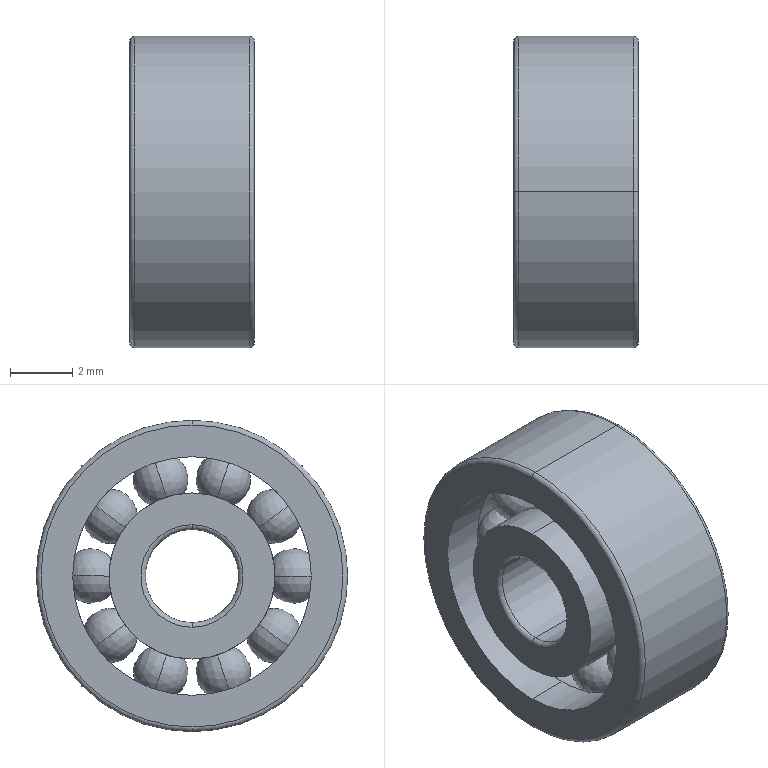Part | SolidWorks | features Revolution 3, CirPattern 1, Fillet 1 | 1 solid | 77 faces | box 4 x 10 x 10 mm | volume 208.039 mm3 | torus 41 | sphere 20 | cylinder 12 | plane 4 | commonest cylinder face diameters 5.333 x4 7.667 x4 3 x2 10 x2